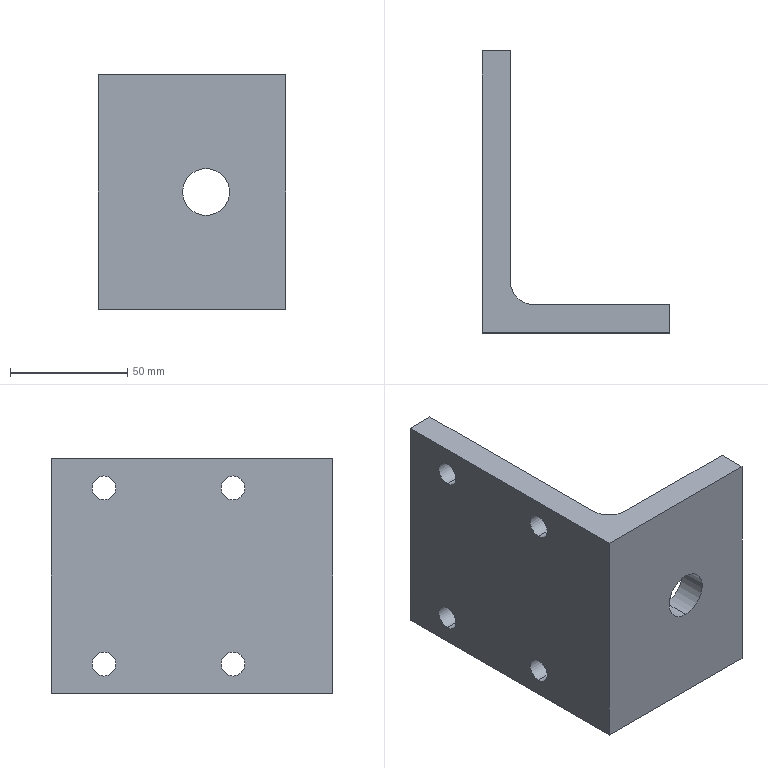Part | SolidWorks | features Extrusion 1, HoleWzd 1, ICE 1 | 1 solid | 19 faces | box 80 x 120 x 100 mm | volume 220054 mm3 | cylinder 11 | plane 8 | commonest cylinder face diameters 10.2 x8 20 x3
STEP:
#1=CARTESIAN_POINT('',(46.,-120.,40.));
#2=VERTEX_POINT('',#1);
#3=CARTESIAN_POINT('',(46.,-120.,60.));
#4=VERTEX_POINT('',#3);
#5=CARTESIAN_POINT('',(46.,-120.,50.));
#6=DIRECTION('',(0.,1.,0.));
#7=DIRECTION('',(0.,0.,1.));
#8=AXIS2_PLACEMENT_3D('',#5,#6,#7);
#9=CIRCLE('',#8,10.);
#10=EDGE_CURVE('',#2,#4,#9,.T.);
#11=ORIENTED_EDGE('',*,*,#10,.F.);
#12=CARTESIAN_POINT('',(46.,-108.,40.));
#13=VERTEX_POINT('',#12);
#14=CARTESIAN_POINT('',(46.,-208.,40.));
#15=DIRECTION('',(0.,1.,0.));
#16=VECTOR('',#15,1000.);
#17=LINE('',#14,#16);
#18=EDGE_CURVE('',#2,#13,#17,.T.);
#19=ORIENTED_EDGE('',*,*,#18,.T.);
#20=CARTESIAN_POINT('',(46.,-108.,60.));
#21=VERTEX_POINT('',#20);
#22=CARTESIAN_POINT('',(46.,-108.,50.));
#23=DIRECTION('',(0.,1.,0.));
#24=DIRECTION('',(0.,0.,1.));
#25=AXIS2_PLACEMENT_3D('',#22,#23,#24);
#26=CIRCLE('',#25,10.);
#27=EDGE_CURVE('',#13,#21,#26,.T.);
#28=ORIENTED_EDGE('',*,*,#27,.T.);
#29=CARTESIAN_POINT('',(46.,-208.,60.));
#30=DIRECTION('',(0.,1.,0.));
#31=VECTOR('',#30,1000.);
#32=LINE('',#29,#31);
#33=EDGE_CURVE('',#4,#21,#32,.T.);
#34=ORIENTED_EDGE('',*,*,#33,.F.);
#35=EDGE_LOOP('',(#11,#19,#28,#34));
#36=FACE_OUTER_BOUND('',#35,.T.);
#37=CARTESIAN_POINT('',(46.,-208.,50.));
#38=DIRECTION('',(0.,1.,0.));
#39=DIRECTION('',(0.,0.,1.));
#40=AXIS2_PLACEMENT_3D('',#37,#38,#39);
#41=CYLINDRICAL_SURFACE('',#40,10.);
#42=ADVANCED_FACE('',(#36),#41,.F.);
#43=CARTESIAN_POINT('',(0.,-22.5,92.6));
#44=VERTEX_POINT('',#43);
#45=CARTESIAN_POINT('',(0.,-22.5,82.4));
#46=VERTEX_POINT('',#45);
#47=CARTESIAN_POINT('',(0.,-22.5,87.5));
#48=DIRECTION('',(1.,0.,0.));
#49=DIRECTION('',(0.,1.,0.));
#50=AXIS2_PLACEMENT_3D('',#47,#48,#49);
#51=CIRCLE('',#50,5.1);
#52=EDGE_CURVE('',#44,#46,#51,.T.);
#53=ORIENTED_EDGE('',*,*,#52,.F.);
#54=CARTESIAN_POINT('',(12.,-22.5,92.6));
#55=VERTEX_POINT('',#54);
#56=CARTESIAN_POINT('',(12.,-22.5,92.6));
#57=DIRECTION('',(1.,0.,0.));
#58=VECTOR('',#57,1000.);
#59=LINE('',#56,#58);
#60=EDGE_CURVE('',#44,#55,#59,.T.);
#61=ORIENTED_EDGE('',*,*,#60,.T.);
#62=CARTESIAN_POINT('',(12.,-22.5,82.4));
#63=VERTEX_POINT('',#62);
#64=CARTESIAN_POINT('',(12.,-22.5,87.5));
#65=DIRECTION('',(1.,0.,0.));
#66=DIRECTION('',(0.,0.,-1.));
#67=AXIS2_PLACEMENT_3D('',#64,#65,#66);
#68=CIRCLE('',#67,5.1);
#69=EDGE_CURVE('',#55,#63,#68,.T.);
#70=ORIENTED_EDGE('',*,*,#69,.T.);
#71=CARTESIAN_POINT('',(12.,-22.5,82.4));
#72=DIRECTION('',(1.,0.,0.));
#73=VECTOR('',#72,1000.);
#74=LINE('',#71,#73);
#75=EDGE_CURVE('',#46,#63,#74,.T.);
#76=ORIENTED_EDGE('',*,*,#75,.F.);
#77=EDGE_LOOP('',(#53,#61,#70,#76));
#78=FACE_OUTER_BOUND('',#77,.T.);
#79=CARTESIAN_POINT('',(12.,-22.5,87.5));
#80=DIRECTION('',(1.,0.,0.));
#81=DIRECTION('',(0.,0.,-1.));
#82=AXIS2_PLACEMENT_3D('',#79,#80,#81);
#83=CYLINDRICAL_SURFACE('',#82,5.1);
#84=ADVANCED_FACE('',(#78),#83,.F.);
#85=CARTESIAN_POINT('',(0.,-22.5,17.6));
#86=VERTEX_POINT('',#85);
#87=CARTESIAN_POINT('',(0.,-22.5,7.4));
#88=VERTEX_POINT('',#87);
#89=CARTESIAN_POINT('',(0.,-22.5,12.5));
#90=DIRECTION('',(1.,0.,0.));
#91=DIRECTION('',(0.,1.,0.));
#92=AXIS2_PLACEMENT_3D('',#89,#90,#91);
#93=CIRCLE('',#92,5.1);
#94=EDGE_CURVE('',#86,#88,#93,.T.);
#95=ORIENTED_EDGE('',*,*,#94,.F.);
#96=CARTESIAN_POINT('',(12.,-22.5,17.6));
#97=VERTEX_POINT('',#96);
#98=CARTESIAN_POINT('',(12.,-22.5,17.6));
#99=DIRECTION('',(1.,0.,0.));
#100=VECTOR('',#99,1000.);
#101=LINE('',#98,#100);
#102=EDGE_CURVE('',#86,#97,#101,.T.);
#103=ORIENTED_EDGE('',*,*,#102,.T.);
#104=CARTESIAN_POINT('',(12.,-22.5,7.4));
#105=VERTEX_POINT('',#104);
#106=CARTESIAN_POINT('',(12.,-22.5,12.5));
#107=DIRECTION('',(1.,0.,0.));
#108=DIRECTION('',(0.,0.,-1.));
#109=AXIS2_PLACEMENT_3D('',#106,#107,#108);
#110=CIRCLE('',#109,5.1);
#111=EDGE_CURVE('',#97,#105,#110,.T.);
#112=ORIENTED_EDGE('',*,*,#111,.T.);
#113=CARTESIAN_POINT('',(12.,-22.5,7.4));
#114=DIRECTION('',(1.,0.,0.));
#115=VECTOR('',#114,1000.);
#116=LINE('',#113,#115);
#117=EDGE_CURVE('',#88,#105,#116,.T.);
#118=ORIENTED_EDGE('',*,*,#117,.F.);
#119=EDGE_LOOP('',(#95,#103,#112,#118));
#120=FACE_OUTER_BOUND('',#119,.T.);
#121=CARTESIAN_POINT('',(12.,-22.5,12.5));
#122=DIRECTION('',(1.,0.,0.));
#123=DIRECTION('',(0.,0.,-1.));
#124=AXIS2_PLACEMENT_3D('',#121,#122,#123);
#125=CYLINDRICAL_SURFACE('',#124,5.1);
#126=ADVANCED_FACE('',(#120),#125,.F.);
#127=CARTESIAN_POINT('',(0.,-77.5,17.6));
#128=VERTEX_POINT('',#127);
#129=CARTESIAN_POINT('',(0.,-77.5,7.4));
#130=VERTEX_POINT('',#129);
#131=CARTESIAN_POINT('',(0.,-77.5,12.5));
#132=DIRECTION('',(1.,0.,0.));
#133=DIRECTION('',(0.,1.,0.));
#134=AXIS2_PLACEMENT_3D('',#131,#132,#133);
#135=CIRCLE('',#134,5.1);
#136=EDGE_CURVE('',#128,#130,#135,.T.);
#137=ORIENTED_EDGE('',*,*,#136,.F.);
#138=CARTESIAN_POINT('',(12.,-77.5,17.6));
#139=VERTEX_POINT('',#138);
#140=CARTESIAN_POINT('',(12.,-77.5,17.6));
#141=DIRECTION('',(1.,0.,0.));
#142=VECTOR('',#141,1000.);
#143=LINE('',#140,#142);
#144=EDGE_CURVE('',#128,#139,#143,.T.);
#145=ORIENTED_EDGE('',*,*,#144,.T.);
#146=CARTESIAN_POINT('',(12.,-77.5,7.4));
#147=VERTEX_POINT('',#146);
#148=CARTESIAN_POINT('',(12.,-77.5,12.5));
#149=DIRECTION('',(1.,0.,0.));
#150=DIRECTION('',(0.,0.,-1.));
#151=AXIS2_PLACEMENT_3D('',#148,#149,#150);
#152=CIRCLE('',#151,5.1);
#153=EDGE_CURVE('',#139,#147,#152,.T.);
#154=ORIENTED_EDGE('',*,*,#153,.T.);
#155=CARTESIAN_POINT('',(12.,-77.5,7.4));
#156=DIRECTION('',(1.,0.,0.));
#157=VECTOR('',#156,1000.);
#158=LINE('',#155,#157);
#159=EDGE_CURVE('',#130,#147,#158,.T.);
#160=ORIENTED_EDGE('',*,*,#159,.F.);
#161=EDGE_LOOP('',(#137,#145,#154,#160));
#162=FACE_OUTER_BOUND('',#161,.T.);
#163=CARTESIAN_POINT('',(12.,-77.5,12.5));
#164=DIRECTION('',(1.,0.,0.));
#165=DIRECTION('',(0.,0.,-1.));
#166=AXIS2_PLACEMENT_3D('',#163,#164,#165);
#167=CYLINDRICAL_SURFACE('',#166,5.1);
#168=ADVANCED_FACE('',(#162),#167,.F.);
#169=CARTESIAN_POINT('',(0.,-77.5,92.6));
#170=VERTEX_POINT('',#169);
#171=CARTESIAN_POINT('',(0.,-77.5,82.4));
#172=VERTEX_POINT('',#171);
#173=CARTESIAN_POINT('',(0.,-77.5,87.5));
#174=DIRECTION('',(1.,0.,0.));
#175=DIRECTION('',(0.,1.,0.));
#176=AXIS2_PLACEMENT_3D('',#173,#174,#175);
#177=CIRCLE('',#176,5.1);
#178=EDGE_CURVE('',#170,#172,#177,.T.);
#179=ORIENTED_EDGE('',*,*,#178,.F.);
#180=CARTESIAN_POINT('',(12.,-77.5,92.6));
#181=VERTEX_POINT('',#180);
#182=CARTESIAN_POINT('',(12.,-77.5,92.6));
#183=DIRECTION('',(1.,0.,0.));
#184=VECTOR('',#183,1000.);
#185=LINE('',#182,#184);
#186=EDGE_CURVE('',#170,#181,#185,.T.);
#187=ORIENTED_EDGE('',*,*,#186,.T.);
#188=CARTESIAN_POINT('',(12.,-77.5,82.4));
#189=VERTEX_POINT('',#188);
#190=CARTESIAN_POINT('',(12.,-77.5,87.5));
#191=DIRECTION('',(1.,0.,0.));
#192=DIRECTION('',(0.,0.,-1.));
#193=AXIS2_PLACEMENT_3D('',#190,#191,#192);
#194=CIRCLE('',#193,5.1);
#195=EDGE_CURVE('',#181,#189,#194,.T.);
#196=ORIENTED_EDGE('',*,*,#195,.T.);
#197=CARTESIAN_POINT('',(12.,-77.5,82.4));
#198=DIRECTION('',(1.,0.,0.));
#199=VECTOR('',#198,1000.);
#200=LINE('',#197,#199);
#201=EDGE_CURVE('',#172,#189,#200,.T.);
#202=ORIENTED_EDGE('',*,*,#201,.F.);
#203=EDGE_LOOP('',(#179,#187,#196,#202));
#204=FACE_OUTER_BOUND('',#203,.T.);
#205=CARTESIAN_POINT('',(12.,-77.5,87.5));
#206=DIRECTION('',(1.,0.,0.));
#207=DIRECTION('',(0.,0.,-1.));
#208=AXIS2_PLACEMENT_3D('',#205,#206,#207);
#209=CYLINDRICAL_SURFACE('',#208,5.1);
#210=ADVANCED_FACE('',(#204),#209,.F.);
#211=CARTESIAN_POINT('',(12.,-22.5,87.5));
#212=DIRECTION('',(1.,0.,0.));
#213=DIRECTION('',(0.,0.,-1.));
#214=AXIS2_PLACEMENT_3D('',#211,#212,#213);
#215=CIRCLE('',#214,5.1);
#216=EDGE_CURVE('',#63,#55,#215,.T.);
#217=ORIENTED_EDGE('',*,*,#216,.F.);
#218=ORIENTED_EDGE('',*,*,#69,.F.);
#219=EDGE_LOOP('',(#217,#218));
#220=FACE_BOUND('',#219,.T.);
#221=CARTESIAN_POINT('',(12.,-22.5,12.5));
#222=DIRECTION('',(1.,0.,0.));
#223=DIRECTION('',(0.,0.,-1.));
#224=AXIS2_PLACEMENT_3D('',#221,#222,#223);
#225=CIRCLE('',#224,5.1);
#226=EDGE_CURVE('',#105,#97,#225,.T.);
#227=ORIENTED_EDGE('',*,*,#226,.F.);
#228=ORIENTED_EDGE('',*,*,#111,.F.);
#229=EDGE_LOOP('',(#227,#228));
#230=FACE_BOUND('',#229,.T.);
#231=CARTESIAN_POINT('',(12.,-77.5,12.5));
#232=DIRECTION('',(1.,0.,0.));
#233=DIRECTION('',(0.,0.,-1.));
#234=AXIS2_PLACEMENT_3D('',#231,#232,#233);
#235=CIRCLE('',#234,5.1);
#236=EDGE_CURVE('',#147,#139,#235,.T.);
#237=ORIENTED_EDGE('',*,*,#236,.F.);
#238=ORIENTED_EDGE('',*,*,#153,.F.);
#239=EDGE_LOOP('',(#237,#238));
#240=FACE_BOUND('',#239,.T.);
#241=CARTESIAN_POINT('',(12.,-77.5,87.5));
#242=DIRECTION('',(1.,0.,0.));
#243=DIRECTION('',(0.,0.,-1.));
#244=AXIS2_PLACEMENT_3D('',#241,#242,#243);
#245=CIRCLE('',#244,5.1);
#246=EDGE_CURVE('',#189,#181,#245,.T.);
#247=ORIENTED_EDGE('',*,*,#246,.F.);
#248=ORIENTED_EDGE('',*,*,#195,.F.);
#249=EDGE_LOOP('',(#247,#248));
#250=FACE_BOUND('',#249,.T.);
#251=CARTESIAN_POINT('',(12.,0.,0.));
#252=VERTEX_POINT('',#251);
#253=CARTESIAN_POINT('',(12.,-98.,0.));
#254=VERTEX_POINT('',#253);
#255=CARTESIAN_POINT('',(12.,0.,0.));
#256=DIRECTION('',(0.,-1.,0.));
#257=VECTOR('',#256,1000.);
#258=LINE('',#255,#257);
#259=EDGE_CURVE('',#252,#254,#258,.T.);
#260=ORIENTED_EDGE('',*,*,#259,.F.);
#261=CARTESIAN_POINT('',(12.,0.,100.));
#262=VERTEX_POINT('',#261);
#263=CARTESIAN_POINT('',(12.,0.,100.));
#264=DIRECTION('',(0.,0.,-1.));
#265=VECTOR('',#264,1000.);
#266=LINE('',#263,#265);
#267=EDGE_CURVE('',#262,#252,#266,.T.);
#268=ORIENTED_EDGE('',*,*,#267,.F.);
#269=CARTESIAN_POINT('',(12.,-98.,100.));
#270=VERTEX_POINT('',#269);
#271=CARTESIAN_POINT('',(12.,0.,100.));
#272=DIRECTION('',(0.,-1.,0.));
#273=VECTOR('',#272,1000.);
#274=LINE('',#271,#273);
#275=EDGE_CURVE('',#262,#270,#274,.T.);
#276=ORIENTED_EDGE('',*,*,#275,.T.);
#277=CARTESIAN_POINT('',(12.,-98.,100.));
#278=DIRECTION('',(0.,0.,-1.));
#279=VECTOR('',#278,1000.);
#280=LINE('',#277,#279);
#281=EDGE_CURVE('',#270,#254,#280,.T.);
#282=ORIENTED_EDGE('',*,*,#281,.T.);
#283=EDGE_LOOP('',(#260,#268,#276,#282));
#284=FACE_OUTER_BOUND('',#283,.T.);
#285=CARTESIAN_POINT('',(12.,0.,100.));
#286=DIRECTION('',(1.,0.,0.));
#287=DIRECTION('',(0.,1.,0.));
#288=AXIS2_PLACEMENT_3D('',#285,#286,#287);
#289=PLANE('',#288);
#290=ADVANCED_FACE('',(#220,#230,#240,#250,#284),#289,.T.);
#291=CARTESIAN_POINT('',(0.,0.,0.));
#292=VERTEX_POINT('',#291);
#293=CARTESIAN_POINT('',(12.,0.,0.));
#294=DIRECTION('',(-1.,0.,0.));
#295=VECTOR('',#294,1000.);
#296=LINE('',#293,#295);
#297=EDGE_CURVE('',#252,#292,#296,.T.);
#298=ORIENTED_EDGE('',*,*,#297,.T.);
#299=CARTESIAN_POINT('',(0.,0.,100.));
#300=VERTEX_POINT('',#299);
#301=CARTESIAN_POINT('',(0.,0.,100.));
#302=DIRECTION('',(0.,0.,-1.));
#303=VECTOR('',#302,1000.);
#304=LINE('',#301,#303);
#305=EDGE_CURVE('',#300,#292,#304,.T.);
#306=ORIENTED_EDGE('',*,*,#305,.F.);
#307=CARTESIAN_POINT('',(12.,0.,100.));
#308=DIRECTION('',(-1.,0.,0.));
#309=VECTOR('',#308,1000.);
#310=LINE('',#307,#309);
#311=EDGE_CURVE('',#262,#300,#310,.T.);
#312=ORIENTED_EDGE('',*,*,#311,.F.);
#313=ORIENTED_EDGE('',*,*,#267,.T.);
#314=EDGE_LOOP('',(#298,#306,#312,#313));
#315=FACE_OUTER_BOUND('',#314,.T.);
#316=CARTESIAN_POINT('',(12.,0.,100.));
#317=DIRECTION('',(0.,-1.,0.));
#318=DIRECTION('',(1.,0.,0.));
#319=AXIS2_PLACEMENT_3D('',#316,#317,#318);
#320=PLANE('',#319);
#321=ADVANCED_FACE('',(#315),#320,.F.);
#322=CARTESIAN_POINT('',(0.,-22.5,87.5));
#323=DIRECTION('',(1.,0.,0.));
#324=DIRECTION('',(0.,1.,0.));
#325=AXIS2_PLACEMENT_3D('',#322,#323,#324);
#326=CIRCLE('',#325,5.1);
#327=EDGE_CURVE('',#46,#44,#326,.T.);
#328=ORIENTED_EDGE('',*,*,#327,.T.);
#329=ORIENTED_EDGE('',*,*,#52,.T.);
#330=EDGE_LOOP('',(#328,#329));
#331=FACE_BOUND('',#330,.T.);
#332=CARTESIAN_POINT('',(0.,-22.5,12.5));
#333=DIRECTION('',(1.,0.,0.));
#334=DIRECTION('',(0.,1.,0.));
#335=AXIS2_PLACEMENT_3D('',#332,#333,#334);
#336=CIRCLE('',#335,5.1);
#337=EDGE_CURVE('',#88,#86,#336,.T.);
#338=ORIENTED_EDGE('',*,*,#337,.T.);
#339=ORIENTED_EDGE('',*,*,#94,.T.);
#340=EDGE_LOOP('',(#338,#339));
#341=FACE_BOUND('',#340,.T.);
#342=CARTESIAN_POINT('',(0.,-77.5,12.5));
#343=DIRECTION('',(1.,0.,0.));
#344=DIRECTION('',(0.,1.,0.));
#345=AXIS2_PLACEMENT_3D('',#342,#343,#344);
#346=CIRCLE('',#345,5.1);
#347=EDGE_CURVE('',#130,#128,#346,.T.);
#348=ORIENTED_EDGE('',*,*,#347,.T.);
#349=ORIENTED_EDGE('',*,*,#136,.T.);
#350=EDGE_LOOP('',(#348,#349));
#351=FACE_BOUND('',#350,.T.);
#352=CARTESIAN_POINT('',(0.,-77.5,87.5));
#353=DIRECTION('',(1.,0.,0.));
#354=DIRECTION('',(0.,1.,0.));
#355=AXIS2_PLACEMENT_3D('',#352,#353,#354);
#356=CIRCLE('',#355,5.1);
#357=EDGE_CURVE('',#172,#170,#356,.T.);
#358=ORIENTED_EDGE('',*,*,#357,.T.);
#359=ORIENTED_EDGE('',*,*,#178,.T.);
#360=EDGE_LOOP('',(#358,#359));
#361=FACE_BOUND('',#360,.T.);
#362=CARTESIAN_POINT('',(0.,-120.,0.));
#363=VERTEX_POINT('',#362);
#364=CARTESIAN_POINT('',(0.,0.,0.));
#365=DIRECTION('',(0.,-1.,0.));
#366=VECTOR('',#365,1000.);
#367=LINE('',#364,#366);
#368=EDGE_CURVE('',#292,#363,#367,.T.);
#369=ORIENTED_EDGE('',*,*,#368,.T.);
#370=CARTESIAN_POINT('',(0.,-120.,100.));
#371=VERTEX_POINT('',#370);
#372=CARTESIAN_POINT('',(0.,-120.,100.));
#373=DIRECTION('',(0.,0.,-1.));
#374=VECTOR('',#373,1000.);
#375=LINE('',#372,#374);
#376=EDGE_CURVE('',#371,#363,#375,.T.);
#377=ORIENTED_EDGE('',*,*,#376,.F.);
#378=CARTESIAN_POINT('',(0.,0.,100.));
#379=DIRECTION('',(0.,-1.,0.));
#380=VECTOR('',#379,1000.);
#381=LINE('',#378,#380);
#382=EDGE_CURVE('',#300,#371,#381,.T.);
#383=ORIENTED_EDGE('',*,*,#382,.F.);
#384=ORIENTED_EDGE('',*,*,#305,.T.);
#385=EDGE_LOOP('',(#369,#377,#383,#384));
#386=FACE_OUTER_BOUND('',#385,.T.);
#387=CARTESIAN_POINT('',(0.,0.,100.));
#388=DIRECTION('',(1.,0.,0.));
#389=DIRECTION('',(0.,1.,0.));
#390=AXIS2_PLACEMENT_3D('',#387,#388,#389);
#391=PLANE('',#390);
#392=ADVANCED_FACE('',(#331,#341,#351,#361,#386),#391,.F.);
#393=CARTESIAN_POINT('',(46.,-120.,50.));
#394=DIRECTION('',(0.,1.,0.));
#395=DIRECTION('',(0.,0.,1.));
#396=AXIS2_PLACEMENT_3D('',#393,#394,#395);
#397=CIRCLE('',#396,10.);
#398=EDGE_CURVE('',#4,#2,#397,.T.);
#399=ORIENTED_EDGE('',*,*,#398,.T.);
#400=ORIENTED_EDGE('',*,*,#10,.T.);
#401=EDGE_LOOP('',(#399,#400));
#402=FACE_BOUND('',#401,.T.);
#403=CARTESIAN_POINT('',(80.,-120.,0.));
#404=VERTEX_POINT('',#403);
#405=CARTESIAN_POINT('',(0.,-120.,0.));
#406=DIRECTION('',(1.,0.,0.));
#407=VECTOR('',#406,1000.);
#408=LINE('',#405,#407);
#409=EDGE_CURVE('',#363,#404,#408,.T.);
#410=ORIENTED_EDGE('',*,*,#409,.T.);
#411=CARTESIAN_POINT('',(80.,-120.,100.));
#412=VERTEX_POINT('',#411);
#413=CARTESIAN_POINT('',(80.,-120.,100.));
#414=DIRECTION('',(0.,0.,-1.));
#415=VECTOR('',#414,1000.);
#416=LINE('',#413,#415);
#417=EDGE_CURVE('',#412,#404,#416,.T.);
#418=ORIENTED_EDGE('',*,*,#417,.F.);
#419=CARTESIAN_POINT('',(0.,-120.,100.));
#420=DIRECTION('',(1.,0.,0.));
#421=VECTOR('',#420,1000.);
#422=LINE('',#419,#421);
#423=EDGE_CURVE('',#371,#412,#422,.T.);
#424=ORIENTED_EDGE('',*,*,#423,.F.);
#425=ORIENTED_EDGE('',*,*,#376,.T.);
#426=EDGE_LOOP('',(#410,#418,#424,#425));
#427=FACE_OUTER_BOUND('',#426,.T.);
#428=CARTESIAN_POINT('',(0.,-120.,100.));
#429=DIRECTION('',(0.,1.,0.));
#430=DIRECTION('',(0.,0.,1.));
#431=AXIS2_PLACEMENT_3D('',#428,#429,#430);
#432=PLANE('',#431);
#433=ADVANCED_FACE('',(#402,#427),#432,.F.);
#434=CARTESIAN_POINT('',(80.,-108.,0.));
#435=VERTEX_POINT('',#434);
#436=CARTESIAN_POINT('',(80.,-108.,0.));
#437=DIRECTION('',(0.,-1.,0.));
#438=VECTOR('',#437,1000.);
#439=LINE('',#436,#438);
#440=EDGE_CURVE('',#435,#404,#439,.T.);
#441=ORIENTED_EDGE('',*,*,#440,.F.);
#442=CARTESIAN_POINT('',(80.,-108.,100.));
#443=VERTEX_POINT('',#442);
#444=CARTESIAN_POINT('',(80.,-108.,100.));
#445=DIRECTION('',(0.,0.,-1.));
#446=VECTOR('',#445,1000.);
#447=LINE('',#444,#446);
#448=EDGE_CURVE('',#443,#435,#447,.T.);
#449=ORIENTED_EDGE('',*,*,#448,.F.);
#450=CARTESIAN_POINT('',(80.,-108.,100.));
#451=DIRECTION('',(0.,-1.,0.));
#452=VECTOR('',#451,1000.);
#453=LINE('',#450,#452);
#454=EDGE_CURVE('',#443,#412,#453,.T.);
#455=ORIENTED_EDGE('',*,*,#454,.T.);
#456=ORIENTED_EDGE('',*,*,#417,.T.);
#457=EDGE_LOOP('',(#441,#449,#455,#456));
#458=FACE_OUTER_BOUND('',#457,.T.);
#459=CARTESIAN_POINT('',(80.,-108.,100.));
#460=DIRECTION('',(1.,0.,0.));
#461=DIRECTION('',(0.,0.,-1.));
#462=AXIS2_PLACEMENT_3D('',#459,#460,#461);
#463=PLANE('',#462);
#464=ADVANCED_FACE('',(#458),#463,.T.);
#465=CARTESIAN_POINT('',(46.,-108.,50.));
#466=DIRECTION('',(0.,1.,0.));
#467=DIRECTION('',(0.,0.,1.));
#468=AXIS2_PLACEMENT_3D('',#465,#466,#467);
#469=CIRCLE('',#468,10.);
#470=EDGE_CURVE('',#21,#13,#469,.T.);
#471=ORIENTED_EDGE('',*,*,#470,.F.);
#472=ORIENTED_EDGE('',*,*,#27,.F.);
#473=EDGE_LOOP('',(#471,#472));
#474=FACE_BOUND('',#473,.T.);
#475=CARTESIAN_POINT('',(22.,-108.,0.));
#476=VERTEX_POINT('',#475);
#477=CARTESIAN_POINT('',(22.,-108.,0.));
#478=DIRECTION('',(1.,0.,0.));
#479=VECTOR('',#478,1000.);
#480=LINE('',#477,#479);
#481=EDGE_CURVE('',#476,#435,#480,.T.);
#482=ORIENTED_EDGE('',*,*,#481,.F.);
#483=CARTESIAN_POINT('',(22.,-108.,100.));
#484=VERTEX_POINT('',#483);
#485=CARTESIAN_POINT('',(22.,-108.,100.));
#486=DIRECTION('',(0.,0.,-1.));
#487=VECTOR('',#486,1000.);
#488=LINE('',#485,#487);
#489=EDGE_CURVE('',#484,#476,#488,.T.);
#490=ORIENTED_EDGE('',*,*,#489,.F.);
#491=CARTESIAN_POINT('',(22.,-108.,100.));
#492=DIRECTION('',(1.,0.,0.));
#493=VECTOR('',#492,1000.);
#494=LINE('',#491,#493);
#495=EDGE_CURVE('',#484,#443,#494,.T.);
#496=ORIENTED_EDGE('',*,*,#495,.T.);
#497=ORIENTED_EDGE('',*,*,#448,.T.);
#498=EDGE_LOOP('',(#482,#490,#496,#497));
#499=FACE_OUTER_BOUND('',#498,.T.);
#500=CARTESIAN_POINT('',(22.,-108.,100.));
#501=DIRECTION('',(0.,1.,0.));
#502=DIRECTION('',(0.,0.,1.));
#503=AXIS2_PLACEMENT_3D('',#500,#501,#502);
#504=PLANE('',#503);
#505=ADVANCED_FACE('',(#474,#499),#504,.T.);
#506=CARTESIAN_POINT('',(22.,-98.,0.));
#507=DIRECTION('',(0.,0.,1.));
#508=DIRECTION('',(1.,0.,0.));
#509=AXIS2_PLACEMENT_3D('',#506,#507,#508);
#510=CIRCLE('',#509,10.);
#511=EDGE_CURVE('',#254,#476,#510,.T.);
#512=ORIENTED_EDGE('',*,*,#511,.F.);
#513=ORIENTED_EDGE('',*,*,#281,.F.);
#514=CARTESIAN_POINT('',(22.,-98.,100.));
#515=DIRECTION('',(0.,0.,1.));
#516=DIRECTION('',(1.,0.,0.));
#517=AXIS2_PLACEMENT_3D('',#514,#515,#516);
#518=CIRCLE('',#517,10.);
#519=EDGE_CURVE('',#270,#484,#518,.T.);
#520=ORIENTED_EDGE('',*,*,#519,.T.);
#521=ORIENTED_EDGE('',*,*,#489,.T.);
#522=EDGE_LOOP('',(#512,#513,#520,#521));
#523=FACE_OUTER_BOUND('',#522,.T.);
#524=CARTESIAN_POINT('',(22.,-98.,100.));
#525=DIRECTION('',(0.,0.,-1.));
#526=DIRECTION('',(-1.,0.,0.));
#527=AXIS2_PLACEMENT_3D('',#524,#525,#526);
#528=CYLINDRICAL_SURFACE('',#527,10.);
#529=ADVANCED_FACE('',(#523),#528,.F.);
#530=ORIENTED_EDGE('',*,*,#275,.F.);
#531=ORIENTED_EDGE('',*,*,#311,.T.);
#532=ORIENTED_EDGE('',*,*,#382,.T.);
#533=ORIENTED_EDGE('',*,*,#423,.T.);
#534=ORIENTED_EDGE('',*,*,#454,.F.);
#535=ORIENTED_EDGE('',*,*,#495,.F.);
#536=ORIENTED_EDGE('',*,*,#519,.F.);
#537=EDGE_LOOP('',(#530,#531,#532,#533,#534,#535,#536));
#538=FACE_OUTER_BOUND('',#537,.T.);
#539=CARTESIAN_POINT('',(22.,-98.,100.));
#540=DIRECTION('',(0.,0.,1.));
#541=DIRECTION('',(1.,0.,0.));
#542=AXIS2_PLACEMENT_3D('',#539,#540,#541);
#543=PLANE('',#542);
#544=ADVANCED_FACE('',(#538),#543,.T.);
#545=ORIENTED_EDGE('',*,*,#259,.T.);
#546=ORIENTED_EDGE('',*,*,#511,.T.);
#547=ORIENTED_EDGE('',*,*,#481,.T.);
#548=ORIENTED_EDGE('',*,*,#440,.T.);
#549=ORIENTED_EDGE('',*,*,#409,.F.);
#550=ORIENTED_EDGE('',*,*,#368,.F.);
#551=ORIENTED_EDGE('',*,*,#297,.F.);
#552=EDGE_LOOP('',(#545,#546,#547,#548,#549,#550,#551));
#553=FACE_OUTER_BOUND('',#552,.T.);
#554=CARTESIAN_POINT('',(22.,-98.,0.));
#555=DIRECTION('',(0.,0.,1.));
#556=DIRECTION('',(1.,0.,0.));
#557=AXIS2_PLACEMENT_3D('',#554,#555,#556);
#558=PLANE('',#557);
#559=ADVANCED_FACE('',(#553),#558,.F.);
#560=ORIENTED_EDGE('',*,*,#186,.F.);
#561=ORIENTED_EDGE('',*,*,#357,.F.);
#562=ORIENTED_EDGE('',*,*,#201,.T.);
#563=ORIENTED_EDGE('',*,*,#246,.T.);
#564=EDGE_LOOP('',(#560,#561,#562,#563));
#565=FACE_OUTER_BOUND('',#564,.T.);
#566=CARTESIAN_POINT('',(12.,-77.5,87.5));
#567=DIRECTION('',(1.,0.,0.));
#568=DIRECTION('',(0.,0.,-1.));
#569=AXIS2_PLACEMENT_3D('',#566,#567,#568);
#570=CYLINDRICAL_SURFACE('',#569,5.1);
#571=ADVANCED_FACE('',(#565),#570,.F.);
#572=ORIENTED_EDGE('',*,*,#144,.F.);
#573=ORIENTED_EDGE('',*,*,#347,.F.);
#574=ORIENTED_EDGE('',*,*,#159,.T.);
#575=ORIENTED_EDGE('',*,*,#236,.T.);
#576=EDGE_LOOP('',(#572,#573,#574,#575));
#577=FACE_OUTER_BOUND('',#576,.T.);
#578=CARTESIAN_POINT('',(12.,-77.5,12.5));
#579=DIRECTION('',(1.,0.,0.));
#580=DIRECTION('',(0.,0.,-1.));
#581=AXIS2_PLACEMENT_3D('',#578,#579,#580);
#582=CYLINDRICAL_SURFACE('',#581,5.1);
#583=ADVANCED_FACE('',(#577),#582,.F.);
#584=ORIENTED_EDGE('',*,*,#102,.F.);
#585=ORIENTED_EDGE('',*,*,#337,.F.);
#586=ORIENTED_EDGE('',*,*,#117,.T.);
#587=ORIENTED_EDGE('',*,*,#226,.T.);
#588=EDGE_LOOP('',(#584,#585,#586,#587));
#589=FACE_OUTER_BOUND('',#588,.T.);
#590=CARTESIAN_POINT('',(12.,-22.5,12.5));
#591=DIRECTION('',(1.,0.,0.));
#592=DIRECTION('',(0.,0.,-1.));
#593=AXIS2_PLACEMENT_3D('',#590,#591,#592);
#594=CYLINDRICAL_SURFACE('',#593,5.1);
#595=ADVANCED_FACE('',(#589),#594,.F.);
#596=ORIENTED_EDGE('',*,*,#60,.F.);
#597=ORIENTED_EDGE('',*,*,#327,.F.);
#598=ORIENTED_EDGE('',*,*,#75,.T.);
#599=ORIENTED_EDGE('',*,*,#216,.T.);
#600=EDGE_LOOP('',(#596,#597,#598,#599));
#601=FACE_OUTER_BOUND('',#600,.T.);
#602=CARTESIAN_POINT('',(12.,-22.5,87.5));
#603=DIRECTION('',(1.,0.,0.));
#604=DIRECTION('',(0.,0.,-1.));
#605=AXIS2_PLACEMENT_3D('',#602,#603,#604);
#606=CYLINDRICAL_SURFACE('',#605,5.1);
#607=ADVANCED_FACE('',(#601),#606,.F.);
#608=ORIENTED_EDGE('',*,*,#18,.F.);
#609=ORIENTED_EDGE('',*,*,#398,.F.);
#610=ORIENTED_EDGE('',*,*,#33,.T.);
#611=ORIENTED_EDGE('',*,*,#470,.T.);
#612=EDGE_LOOP('',(#608,#609,#610,#611));
#613=FACE_OUTER_BOUND('',#612,.T.);
#614=CARTESIAN_POINT('',(46.,-208.,50.));
#615=DIRECTION('',(0.,1.,0.));
#616=DIRECTION('',(0.,0.,1.));
#617=AXIS2_PLACEMENT_3D('',#614,#615,#616);
#618=CYLINDRICAL_SURFACE('',#617,10.);
#619=ADVANCED_FACE('',(#613),#618,.F.);
#620=CLOSED_SHELL('',(#42,#84,#126,#168,#210,#290,#321,#392,#433,#464,#505,#529,#544,#559,#571,#583,#595,#607,#619));
#621=MANIFOLD_SOLID_BREP('',#620);
#622=CARTESIAN_POINT('',(0.,0.,0.));
#623=DIRECTION('',(0.,0.,1.));
#624=DIRECTION('',(1.,0.,0.));
#625=AXIS2_PLACEMENT_3D('',#622,#623,#624);
#626=(LENGTH_UNIT()NAMED_UNIT(*)SI_UNIT(.MILLI.,.METRE.));
#627=UNCERTAINTY_MEASURE_WITH_UNIT(LENGTH_MEASURE(0.00001),#626,'','');
#628=(NAMED_UNIT(*)PLANE_ANGLE_UNIT()SI_UNIT($,.RADIAN.));
#629=(NAMED_UNIT(*)SI_UNIT($,.STERADIAN.)SOLID_ANGLE_UNIT());
#630=(GEOMETRIC_REPRESENTATION_CONTEXT(3)GLOBAL_UNCERTAINTY_ASSIGNED_CONTEXT((#627))GLOBAL_UNIT_ASSIGNED_CONTEXT((#626,#628,#629))REPRESENTATION_CONTEXT('',''));
#631=ADVANCED_BREP_SHAPE_REPRESENTATION('',(#621,#625),#630);